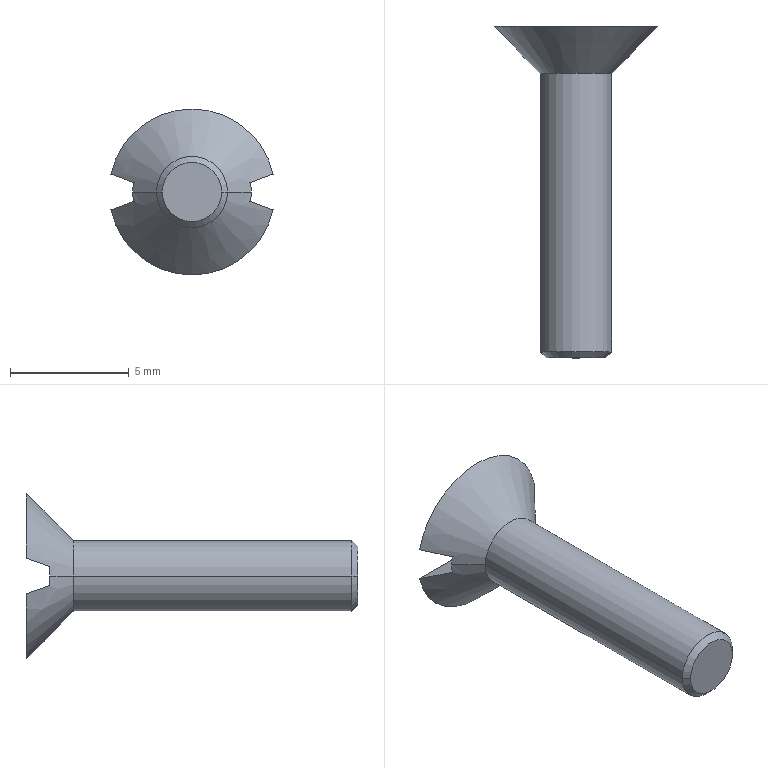Part | SolidWorks | features BaseBody 1 | 1 solid | 12 faces | box 6.837 x 14 x 7 mm | volume 118.937 mm3 | plane 6 | cone 4 | cylinder 2 | commonest cylinder face diameters 3 x2
STEP:
#1=CARTESIAN_POINT('',(-1.25,-12.,0.));
#2=VERTEX_POINT('',#1);
#3=CARTESIAN_POINT('',(1.25,-12.,0.));
#4=VERTEX_POINT('',#3);
#5=CARTESIAN_POINT('',(0.,-12.,0.));
#6=DIRECTION('',(0.,1.,0.));
#7=DIRECTION('',(-1.,0.,0.));
#8=AXIS2_PLACEMENT_3D('',#5,#6,#7);
#9=CIRCLE('',#8,1.25);
#10=EDGE_CURVE('',#2,#4,#9,.T.);
#11=ORIENTED_EDGE('',*,*,#10,.T.);
#12=CARTESIAN_POINT('',(1.5,-11.75,0.));
#13=VERTEX_POINT('',#12);
#14=CARTESIAN_POINT('',(1.375,-11.875,0.));
#15=DIRECTION('',(0.7071,0.7071,0.));
#16=VECTOR('',#15,1000.);
#17=LINE('',#14,#16);
#18=EDGE_CURVE('',#4,#13,#17,.T.);
#19=ORIENTED_EDGE('',*,*,#18,.T.);
#20=CARTESIAN_POINT('',(-1.5,-11.75,0.));
#21=VERTEX_POINT('',#20);
#22=CARTESIAN_POINT('',(0.,-11.75,0.));
#23=DIRECTION('',(0.,-1.,0.));
#24=DIRECTION('',(-1.,0.,0.));
#25=AXIS2_PLACEMENT_3D('',#22,#23,#24);
#26=CIRCLE('',#25,1.5);
#27=EDGE_CURVE('',#13,#21,#26,.T.);
#28=ORIENTED_EDGE('',*,*,#27,.T.);
#29=CARTESIAN_POINT('',(-1.375,-11.875,0.));
#30=DIRECTION('',(-0.7071,0.7071,0.));
#31=VECTOR('',#30,1000.);
#32=LINE('',#29,#31);
#33=EDGE_CURVE('',#2,#21,#32,.T.);
#34=ORIENTED_EDGE('',*,*,#33,.F.);
#35=EDGE_LOOP('',(#11,#19,#28,#34));
#36=FACE_OUTER_BOUND('',#35,.T.);
#37=CARTESIAN_POINT('',(0.,-11.875,0.));
#38=DIRECTION('',(0.,1.,0.));
#39=DIRECTION('',(-1.,0.,0.));
#40=AXIS2_PLACEMENT_3D('',#37,#38,#39);
#41=CONICAL_SURFACE('',#40,1.375,0.7854);
#42=ADVANCED_FACE('',(#36),#41,.T.);
#43=ORIENTED_EDGE('',*,*,#27,.F.);
#44=CARTESIAN_POINT('',(1.5,0.,0.));
#45=VERTEX_POINT('',#44);
#46=CARTESIAN_POINT('',(1.5,0.,0.));
#47=DIRECTION('',(0.,1.,0.));
#48=VECTOR('',#47,1000.);
#49=LINE('',#46,#48);
#50=EDGE_CURVE('',#13,#45,#49,.T.);
#51=ORIENTED_EDGE('',*,*,#50,.T.);
#52=CARTESIAN_POINT('',(-1.5,0.,0.));
#53=VERTEX_POINT('',#52);
#54=CARTESIAN_POINT('',(0.,0.,0.));
#55=DIRECTION('',(0.,1.,0.));
#56=DIRECTION('',(1.,0.,0.));
#57=AXIS2_PLACEMENT_3D('',#54,#55,#56);
#58=CIRCLE('',#57,1.5);
#59=EDGE_CURVE('',#53,#45,#58,.T.);
#60=ORIENTED_EDGE('',*,*,#59,.F.);
#61=CARTESIAN_POINT('',(-1.5,0.,0.));
#62=DIRECTION('',(0.,1.,0.));
#63=VECTOR('',#62,1000.);
#64=LINE('',#61,#63);
#65=EDGE_CURVE('',#21,#53,#64,.T.);
#66=ORIENTED_EDGE('',*,*,#65,.F.);
#67=EDGE_LOOP('',(#43,#51,#60,#66));
#68=FACE_OUTER_BOUND('',#67,.T.);
#69=CARTESIAN_POINT('',(0.,0.,0.));
#70=DIRECTION('',(0.,1.,0.));
#71=DIRECTION('',(-1.,0.,0.));
#72=AXIS2_PLACEMENT_3D('',#69,#70,#71);
#73=CYLINDRICAL_SURFACE('',#72,1.5);
#74=ADVANCED_FACE('',(#68),#73,.T.);
#75=ORIENTED_EDGE('',*,*,#59,.T.);
#76=CARTESIAN_POINT('',(2.5,1.,0.));
#77=VERTEX_POINT('',#76);
#78=CARTESIAN_POINT('',(2.5,1.,0.));
#79=DIRECTION('',(0.7071,0.7071,0.));
#80=VECTOR('',#79,1000.);
#81=LINE('',#78,#80);
#82=EDGE_CURVE('',#45,#77,#81,.T.);
#83=ORIENTED_EDGE('',*,*,#82,.T.);
#84=CARTESIAN_POINT('',(2.468,1.,0.4));
#85=VERTEX_POINT('',#84);
#86=CARTESIAN_POINT('',(0.,1.,0.));
#87=DIRECTION('',(0.,-1.,0.));
#88=DIRECTION('',(-1.,0.,0.));
#89=AXIS2_PLACEMENT_3D('',#86,#87,#88);
#90=CIRCLE('',#89,2.5);
#91=EDGE_CURVE('',#77,#85,#90,.T.);
#92=ORIENTED_EDGE('',*,*,#91,.T.);
#93=CARTESIAN_POINT('',(3.419,2.,0.75));
#94=VERTEX_POINT('',#93);
#95=CARTESIAN_POINT('',(2.468,1.,0.4));
#96=CARTESIAN_POINT('',(2.869,1.419,0.5467));
#97=CARTESIAN_POINT('',(3.419,2.,0.75));
#98=(BOUNDED_CURVE()B_SPLINE_CURVE(2,(#95,#96,#97),.UNSPECIFIED.,.F.,.F.)B_SPLINE_CURVE_WITH_KNOTS((3,3),(0.,0.1424),.UNSPECIFIED.)CURVE()GEOMETRIC_REPRESENTATION_ITEM()RATIONAL_B_SPLINE_CURVE((1.,1.013,1.))REPRESENTATION_ITEM(''));
#99=EDGE_CURVE('',#85,#94,#98,.T.);
#100=ORIENTED_EDGE('',*,*,#99,.T.);
#101=CARTESIAN_POINT('',(-3.419,2.,0.75));
#102=VERTEX_POINT('',#101);
#103=CARTESIAN_POINT('',(0.,2.,0.));
#104=DIRECTION('',(0.,1.,0.));
#105=DIRECTION('',(1.,0.,0.));
#106=AXIS2_PLACEMENT_3D('',#103,#104,#105);
#107=CIRCLE('',#106,3.5);
#108=EDGE_CURVE('',#102,#94,#107,.T.);
#109=ORIENTED_EDGE('',*,*,#108,.F.);
#110=CARTESIAN_POINT('',(-2.468,1.,0.4));
#111=VERTEX_POINT('',#110);
#112=CARTESIAN_POINT('',(-3.419,2.,0.75));
#113=CARTESIAN_POINT('',(-2.869,1.419,0.5467));
#114=CARTESIAN_POINT('',(-2.468,1.,0.4));
#115=(BOUNDED_CURVE()B_SPLINE_CURVE(2,(#112,#113,#114),.UNSPECIFIED.,.F.,.F.)B_SPLINE_CURVE_WITH_KNOTS((3,3),(0.,0.1424),.UNSPECIFIED.)CURVE()GEOMETRIC_REPRESENTATION_ITEM()RATIONAL_B_SPLINE_CURVE((1.,1.013,1.))REPRESENTATION_ITEM(''));
#116=EDGE_CURVE('',#102,#111,#115,.T.);
#117=ORIENTED_EDGE('',*,*,#116,.T.);
#118=CARTESIAN_POINT('',(-2.5,1.,0.));
#119=VERTEX_POINT('',#118);
#120=CARTESIAN_POINT('',(0.,1.,0.));
#121=DIRECTION('',(0.,-1.,0.));
#122=DIRECTION('',(-1.,0.,0.));
#123=AXIS2_PLACEMENT_3D('',#120,#121,#122);
#124=CIRCLE('',#123,2.5);
#125=EDGE_CURVE('',#111,#119,#124,.T.);
#126=ORIENTED_EDGE('',*,*,#125,.T.);
#127=CARTESIAN_POINT('',(-2.5,1.,0.));
#128=DIRECTION('',(-0.7071,0.7071,0.));
#129=VECTOR('',#128,1000.);
#130=LINE('',#127,#129);
#131=EDGE_CURVE('',#53,#119,#130,.T.);
#132=ORIENTED_EDGE('',*,*,#131,.F.);
#133=EDGE_LOOP('',(#75,#83,#92,#100,#109,#117,#126,#132));
#134=FACE_OUTER_BOUND('',#133,.T.);
#135=CARTESIAN_POINT('',(0.,1.,0.));
#136=DIRECTION('',(0.,1.,0.));
#137=DIRECTION('',(-1.,0.,0.));
#138=AXIS2_PLACEMENT_3D('',#135,#136,#137);
#139=CONICAL_SURFACE('',#138,2.5,0.7854);
#140=ADVANCED_FACE('',(#134),#139,.T.);
#141=CARTESIAN_POINT('',(-2.468,1.,-0.4));
#142=VERTEX_POINT('',#141);
#143=CARTESIAN_POINT('',(-3.419,2.,-0.75));
#144=VERTEX_POINT('',#143);
#145=CARTESIAN_POINT('',(-2.468,1.,-0.4));
#146=CARTESIAN_POINT('',(-2.869,1.419,-0.5467));
#147=CARTESIAN_POINT('',(-3.419,2.,-0.75));
#148=(BOUNDED_CURVE()B_SPLINE_CURVE(2,(#145,#146,#147),.UNSPECIFIED.,.F.,.F.)B_SPLINE_CURVE_WITH_KNOTS((3,3),(0.,0.1424),.UNSPECIFIED.)CURVE()GEOMETRIC_REPRESENTATION_ITEM()RATIONAL_B_SPLINE_CURVE((1.,1.013,1.))REPRESENTATION_ITEM(''));
#149=EDGE_CURVE('',#142,#144,#148,.T.);
#150=ORIENTED_EDGE('',*,*,#149,.F.);
#151=CARTESIAN_POINT('',(2.468,1.,-0.4));
#152=VERTEX_POINT('',#151);
#153=CARTESIAN_POINT('',(3.5,1.,-0.4));
#154=DIRECTION('',(-1.,0.,0.));
#155=VECTOR('',#154,1000.);
#156=LINE('',#153,#155);
#157=EDGE_CURVE('',#152,#142,#156,.T.);
#158=ORIENTED_EDGE('',*,*,#157,.F.);
#159=CARTESIAN_POINT('',(3.419,2.,-0.75));
#160=VERTEX_POINT('',#159);
#161=CARTESIAN_POINT('',(3.419,2.,-0.75));
#162=CARTESIAN_POINT('',(2.869,1.419,-0.5467));
#163=CARTESIAN_POINT('',(2.468,1.,-0.4));
#164=(BOUNDED_CURVE()B_SPLINE_CURVE(2,(#161,#162,#163),.UNSPECIFIED.,.F.,.F.)B_SPLINE_CURVE_WITH_KNOTS((3,3),(0.,0.1424),.UNSPECIFIED.)CURVE()GEOMETRIC_REPRESENTATION_ITEM()RATIONAL_B_SPLINE_CURVE((1.,1.013,1.))REPRESENTATION_ITEM(''));
#165=EDGE_CURVE('',#160,#152,#164,.T.);
#166=ORIENTED_EDGE('',*,*,#165,.F.);
#167=CARTESIAN_POINT('',(1.75,2.,-0.75));
#168=DIRECTION('',(1.,0.,0.));
#169=VECTOR('',#168,1000.);
#170=LINE('',#167,#169);
#171=EDGE_CURVE('',#144,#160,#170,.T.);
#172=ORIENTED_EDGE('',*,*,#171,.F.);
#173=EDGE_LOOP('',(#150,#158,#166,#172));
#174=FACE_OUTER_BOUND('',#173,.T.);
#175=CARTESIAN_POINT('',(3.5,2.,-0.75));
#176=DIRECTION('',(0.,-0.3304,-0.9439));
#177=DIRECTION('',(0.,-0.9439,0.3304));
#178=AXIS2_PLACEMENT_3D('',#175,#176,#177);
#179=PLANE('',#178);
#180=ADVANCED_FACE('',(#174),#179,.F.);
#181=ORIENTED_EDGE('',*,*,#116,.F.);
#182=CARTESIAN_POINT('',(1.75,2.,0.75));
#183=DIRECTION('',(-1.,0.,0.));
#184=VECTOR('',#183,1000.);
#185=LINE('',#182,#184);
#186=EDGE_CURVE('',#94,#102,#185,.T.);
#187=ORIENTED_EDGE('',*,*,#186,.F.);
#188=ORIENTED_EDGE('',*,*,#99,.F.);
#189=CARTESIAN_POINT('',(3.5,1.,0.4));
#190=DIRECTION('',(-1.,0.,0.));
#191=VECTOR('',#190,1000.);
#192=LINE('',#189,#191);
#193=EDGE_CURVE('',#85,#111,#192,.T.);
#194=ORIENTED_EDGE('',*,*,#193,.T.);
#195=EDGE_LOOP('',(#181,#187,#188,#194));
#196=FACE_OUTER_BOUND('',#195,.T.);
#197=CARTESIAN_POINT('',(3.5,1.,0.4));
#198=DIRECTION('',(0.,-0.3304,0.9439));
#199=DIRECTION('',(-1.,0.,0.));
#200=AXIS2_PLACEMENT_3D('',#197,#198,#199);
#201=PLANE('',#200);
#202=ADVANCED_FACE('',(#196),#201,.F.);
#203=ORIENTED_EDGE('',*,*,#125,.F.);
#204=ORIENTED_EDGE('',*,*,#193,.F.);
#205=ORIENTED_EDGE('',*,*,#91,.F.);
#206=CARTESIAN_POINT('',(0.,1.,0.));
#207=DIRECTION('',(0.,-1.,0.));
#208=DIRECTION('',(-1.,0.,0.));
#209=AXIS2_PLACEMENT_3D('',#206,#207,#208);
#210=CIRCLE('',#209,2.5);
#211=EDGE_CURVE('',#152,#77,#210,.T.);
#212=ORIENTED_EDGE('',*,*,#211,.F.);
#213=ORIENTED_EDGE('',*,*,#157,.T.);
#214=CARTESIAN_POINT('',(0.,1.,0.));
#215=DIRECTION('',(0.,-1.,0.));
#216=DIRECTION('',(-1.,0.,0.));
#217=AXIS2_PLACEMENT_3D('',#214,#215,#216);
#218=CIRCLE('',#217,2.5);
#219=EDGE_CURVE('',#119,#142,#218,.T.);
#220=ORIENTED_EDGE('',*,*,#219,.F.);
#221=EDGE_LOOP('',(#203,#204,#205,#212,#213,#220));
#222=FACE_OUTER_BOUND('',#221,.T.);
#223=CARTESIAN_POINT('',(3.5,1.,-0.4));
#224=DIRECTION('',(0.,-1.,0.));
#225=DIRECTION('',(0.,0.,-1.));
#226=AXIS2_PLACEMENT_3D('',#223,#224,#225);
#227=PLANE('',#226);
#228=ADVANCED_FACE('',(#222),#227,.F.);
#229=ORIENTED_EDGE('',*,*,#186,.T.);
#230=ORIENTED_EDGE('',*,*,#108,.T.);
#231=EDGE_LOOP('',(#229,#230));
#232=FACE_OUTER_BOUND('',#231,.T.);
#233=CARTESIAN_POINT('',(0.,2.,0.));
#234=DIRECTION('',(0.,1.,0.));
#235=DIRECTION('',(1.,0.,0.));
#236=AXIS2_PLACEMENT_3D('',#233,#234,#235);
#237=PLANE('',#236);
#238=ADVANCED_FACE('',(#232),#237,.T.);
#239=ORIENTED_EDGE('',*,*,#171,.T.);
#240=CARTESIAN_POINT('',(0.,2.,0.));
#241=DIRECTION('',(0.,1.,0.));
#242=DIRECTION('',(1.,0.,0.));
#243=AXIS2_PLACEMENT_3D('',#240,#241,#242);
#244=CIRCLE('',#243,3.5);
#245=EDGE_CURVE('',#160,#144,#244,.T.);
#246=ORIENTED_EDGE('',*,*,#245,.T.);
#247=EDGE_LOOP('',(#239,#246));
#248=FACE_OUTER_BOUND('',#247,.T.);
#249=CARTESIAN_POINT('',(0.,2.,0.));
#250=DIRECTION('',(0.,1.,0.));
#251=DIRECTION('',(1.,0.,0.));
#252=AXIS2_PLACEMENT_3D('',#249,#250,#251);
#253=PLANE('',#252);
#254=ADVANCED_FACE('',(#248),#253,.T.);
#255=ORIENTED_EDGE('',*,*,#10,.F.);
#256=CARTESIAN_POINT('',(0.,-12.,0.));
#257=DIRECTION('',(0.,1.,0.));
#258=DIRECTION('',(-1.,0.,0.));
#259=AXIS2_PLACEMENT_3D('',#256,#257,#258);
#260=CIRCLE('',#259,1.25);
#261=EDGE_CURVE('',#4,#2,#260,.T.);
#262=ORIENTED_EDGE('',*,*,#261,.F.);
#263=EDGE_LOOP('',(#255,#262));
#264=FACE_OUTER_BOUND('',#263,.T.);
#265=CARTESIAN_POINT('',(0.,-12.,0.));
#266=DIRECTION('',(0.,1.,0.));
#267=DIRECTION('',(1.,0.,0.));
#268=AXIS2_PLACEMENT_3D('',#265,#266,#267);
#269=PLANE('',#268);
#270=ADVANCED_FACE('',(#264),#269,.F.);
#271=ORIENTED_EDGE('',*,*,#82,.F.);
#272=CARTESIAN_POINT('',(0.,0.,0.));
#273=DIRECTION('',(0.,1.,0.));
#274=DIRECTION('',(1.,0.,0.));
#275=AXIS2_PLACEMENT_3D('',#272,#273,#274);
#276=CIRCLE('',#275,1.5);
#277=EDGE_CURVE('',#45,#53,#276,.T.);
#278=ORIENTED_EDGE('',*,*,#277,.T.);
#279=ORIENTED_EDGE('',*,*,#131,.T.);
#280=ORIENTED_EDGE('',*,*,#219,.T.);
#281=ORIENTED_EDGE('',*,*,#149,.T.);
#282=ORIENTED_EDGE('',*,*,#245,.F.);
#283=ORIENTED_EDGE('',*,*,#165,.T.);
#284=ORIENTED_EDGE('',*,*,#211,.T.);
#285=EDGE_LOOP('',(#271,#278,#279,#280,#281,#282,#283,#284));
#286=FACE_OUTER_BOUND('',#285,.T.);
#287=CARTESIAN_POINT('',(0.,1.,0.));
#288=DIRECTION('',(0.,1.,0.));
#289=DIRECTION('',(-1.,0.,0.));
#290=AXIS2_PLACEMENT_3D('',#287,#288,#289);
#291=CONICAL_SURFACE('',#290,2.5,0.7854);
#292=ADVANCED_FACE('',(#286),#291,.T.);
#293=ORIENTED_EDGE('',*,*,#50,.F.);
#294=CARTESIAN_POINT('',(0.,-11.75,0.));
#295=DIRECTION('',(0.,-1.,0.));
#296=DIRECTION('',(-1.,0.,0.));
#297=AXIS2_PLACEMENT_3D('',#294,#295,#296);
#298=CIRCLE('',#297,1.5);
#299=EDGE_CURVE('',#21,#13,#298,.T.);
#300=ORIENTED_EDGE('',*,*,#299,.F.);
#301=ORIENTED_EDGE('',*,*,#65,.T.);
#302=ORIENTED_EDGE('',*,*,#277,.F.);
#303=EDGE_LOOP('',(#293,#300,#301,#302));
#304=FACE_OUTER_BOUND('',#303,.T.);
#305=CARTESIAN_POINT('',(0.,0.,0.));
#306=DIRECTION('',(0.,1.,0.));
#307=DIRECTION('',(-1.,0.,0.));
#308=AXIS2_PLACEMENT_3D('',#305,#306,#307);
#309=CYLINDRICAL_SURFACE('',#308,1.5);
#310=ADVANCED_FACE('',(#304),#309,.T.);
#311=ORIENTED_EDGE('',*,*,#18,.F.);
#312=ORIENTED_EDGE('',*,*,#261,.T.);
#313=ORIENTED_EDGE('',*,*,#33,.T.);
#314=ORIENTED_EDGE('',*,*,#299,.T.);
#315=EDGE_LOOP('',(#311,#312,#313,#314));
#316=FACE_OUTER_BOUND('',#315,.T.);
#317=CARTESIAN_POINT('',(0.,-11.875,0.));
#318=DIRECTION('',(0.,1.,0.));
#319=DIRECTION('',(-1.,0.,0.));
#320=AXIS2_PLACEMENT_3D('',#317,#318,#319);
#321=CONICAL_SURFACE('',#320,1.375,0.7854);
#322=ADVANCED_FACE('',(#316),#321,.T.);
#323=CLOSED_SHELL('',(#42,#74,#140,#180,#202,#228,#238,#254,#270,#292,#310,#322));
#324=MANIFOLD_SOLID_BREP('',#323);
#325=CARTESIAN_POINT('',(0.,0.,0.));
#326=DIRECTION('',(0.,0.,1.));
#327=DIRECTION('',(1.,0.,0.));
#328=AXIS2_PLACEMENT_3D('',#325,#326,#327);
#329=(LENGTH_UNIT()NAMED_UNIT(*)SI_UNIT(.MILLI.,.METRE.));
#330=UNCERTAINTY_MEASURE_WITH_UNIT(LENGTH_MEASURE(0.00001),#329,'','');
#331=(NAMED_UNIT(*)PLANE_ANGLE_UNIT()SI_UNIT($,.RADIAN.));
#332=(NAMED_UNIT(*)SI_UNIT($,.STERADIAN.)SOLID_ANGLE_UNIT());
#333=(GEOMETRIC_REPRESENTATION_CONTEXT(3)GLOBAL_UNCERTAINTY_ASSIGNED_CONTEXT((#330))GLOBAL_UNIT_ASSIGNED_CONTEXT((#329,#331,#332))REPRESENTATION_CONTEXT('',''));
#334=ADVANCED_BREP_SHAPE_REPRESENTATION('',(#324,#328),#333);